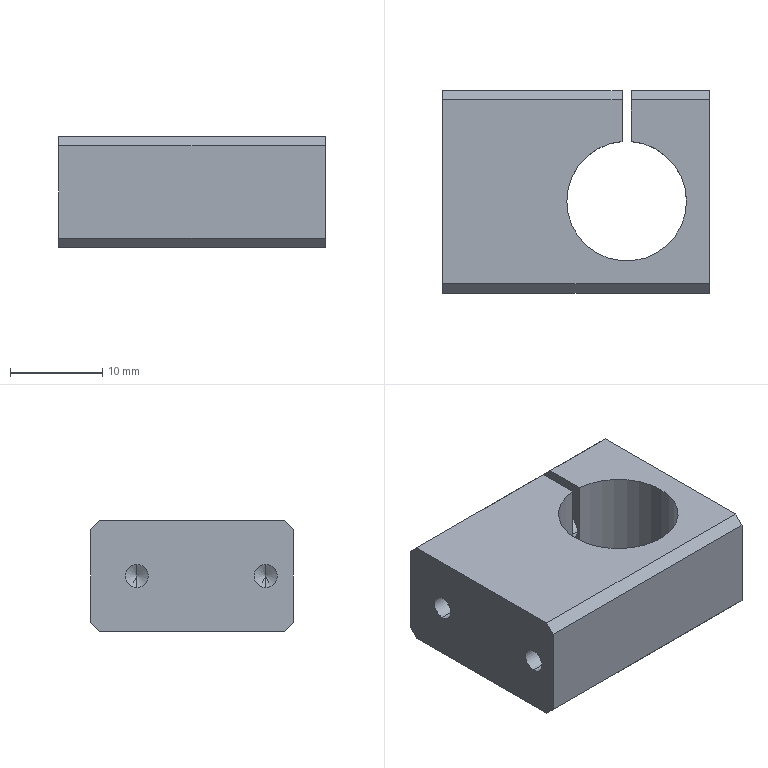NC program | NX | posted with a generic post | part box 29 x 22 x 12 mm
Whole program:
N10 G17 G21 G94 G90
(DRILLING_COPY_1 , TOOL : D6A45)
N12 T01 M6
N14 G54
N16 G17 G0 G90 X7.5 Y0. B0. C0. S5000 M3
N18 G43 Z30. H1
N20 G94 G81 G98 Z-1. F250. R3.
N22 G80
N24 G0 X7.5 Y0. Z30.
N26 M5
(DRILLING_COPY_1_COPY_COPY , TOOL : 2.5ZT)
N28 T12 M6
N30 G54
N32 G17 G0 G90 X7.5 Y0. B0. C0. S2000 M3
N34 G43 Z30. H12
N36 G94 G83 G98 Z-18.251 F150. Q2. R3.
N38 G80
N40 G0 X7.5 Y0. Z30.
N42 M5
(DRILLING_COPY_1_COPY , TOOL : 3.4ZT)
N44 T13 M6
N46 G54
N48 G17 G0 G90 X7.5 Y0. B0. C0. S2000 M3
N50 G43 Z30. H13
N52 G94 G83 G98 Z-10.021 F150. Q2. R3.
N54 G80
N56 G0 X7.5 Y0. Z30.
N58 M5
(HOLE_MILLING_1 , TOOL : D4)
N60 T04 M6
N62 G54
N64 G17 G0 G90 X7.5 Y0. B0. C0. S9500 M3
N66 G43 Z30. H4
N68 Z0.5
N70 G94 G3 X8. Y-0.5 R0.5 F1300.
N72 X8.5 Y0. R0.5
N74 X8.5 Y0. Z0.2 I-1. J0.
N76 X8.5 Y0. Z-0.1 I-1. J0.
N78 X8.5 Y0. Z-0.4 I-1. J0.
N80 X8.5 Y0. Z-0.7 I-1. J0.
N82 X8.5 Y0. Z-1. I-1. J0.
N84 X8.5 Y0. Z-1.3 I-1. J0.
N86 X8.5 Y0. Z-1.6 I-1. J0.
N88 X8.5 Y0. Z-1.9 I-1. J0.
N90 X8.5 Y0. Z-2.2 I-1. J0.
N92 X8.5 Y0. Z-2.5 I-1. J0.
N94 X8.5 Y0. Z-2.8 I-1. J0.
N96 X8.5 Y0. Z-3.1 I-1. J0.
N98 X8.5 Y0. Z-3.4 I-1. J0.
N100 X7.5 Y1. R1.
N102 X8.5 Y0. R-1.
N104 X8. Y0.5 R0.5
N106 X7.5 Y0. R0.5
N108 G0 Z30.
N110 M5
(11_COPY_COPY_COPY_COPY , TOOL : D6A45)
N112 T01 M6
N114 G54
N116 G17 G0 G90 X8.306 Y-0.241 B0. C0. S9500 M3
N118 G43 Z30. H1
N120 Z2.
N122 G94 G1 Z-1. F1000.
N124 X9.241 Y-0.52
N126 G3 X9.541 Y0. R0.6
N128 X7.5 Y2.041 R2.041
N130 X9.541 Y0. R-2.041
N132 X9.241 Y0.52 R0.6
N134 G1 X8.306 Y0.241
N136 Z2.
N138 G0 Z30.
N140 X-10.921 Y7.952
N142 Z2.
N144 G1 Z-1.
N146 X-10.52 Y7.259
N148 G3 X-10.001 Y6.959 R0.6
N150 G1 X10.001
N152 G2 X10.677 Y6.678 R0.957
N154 G1 X11.679 Y5.677
N156 G2 X11.959 Y5.001 R0.988
N158 G1 Y-5.001
N160 G2 X11.679 Y-5.677 R0.988
N162 G1 X10.677 Y-6.678
N164 G2 X10.001 Y-6.959 R0.957
N166 G1 X-10.001
N168 G2 X-10.677 Y-6.678 R0.957
N170 G1 X-11.678 Y-5.677
N172 G2 X-11.959 Y-5.001 R0.957
N174 G1 Y5.001
N176 G2 X-11.678 Y5.677 R0.957
N178 G1 X-10.677 Y6.678
N180 G2 X-10.001 Y6.959 R0.957
N182 G3 X-9.481 Y7.259 R0.6
N184 G1 X-8.961 Y8.159
N186 Z2.
N188 G0 Z30.
N190 M5
(CUTTERCOMP11 , TOOL : 2.3XYD)
N192 T11 M6
N194 G54
N196 G17 G0 G90 X7.5 Y0. B0. C0. S5000 M3
N198 G43 Z30. H11
N200 Z-7.936
N202 G42 G94 G1 X7.578 Y0.062 F850. D11
N204 X7.628 Y0.08 Z-7.957
N206 X7.675 Y0.052 Z-7.979
N208 X7.683 Y0. Z-8.
N210 G2 X7.683 Y0. Z-8.5 I-0.183 J0.
N212 X7.683 Y0. Z-9. I-0.183 J0.
N214 X7.683 Y0. Z-9.5 I-0.183 J0.
N216 X7.683 Y0. Z-10. I-0.183 J0.
N218 X7.683 Y0. Z-10.5 I-0.183 J0.
N220 X7.683 Y0. Z-11. I-0.183 J0.
N222 X7.683 Y0. Z-11.5 I-0.183 J0.
N224 X7.683 Y0. Z-12. I-0.183 J0.
N226 X7.683 Y0. Z-12.5 I-0.183 J0.
N228 X7.683 Y0. Z-13. I-0.183 J0.
N230 X7.683 Y0. Z-13.5 I-0.183 J0.
N232 X7.683 Y0. Z-14. I-0.183 J0.
N234 X7.683 Y0. Z-14.5 I-0.183 J0.
N236 X7.683 Y0. Z-15. I-0.183 J0.
N238 X7.683 Y0. Z-15.5 I-0.183 J0.
N240 X7.683 Y0. Z-16. I-0.183 J0.
N242 X7.683 Y0. Z-16.5 I-0.183 J0.
N244 X7.683 Y0. Z-17. I-0.183 J0.
N246 X7.683 Y0. Z-17.5 I-0.183 J0.
N248 G1 X7.675 Y-0.052 Z-17.521
N250 X7.628 Y-0.08 Z-17.543
N252 X7.578 Y-0.062 Z-17.564
N254 G40
N256 X7.5 Y0.
N258 G0 Z30.
N260 Z-7.913
N262 G42 G1 X7.555 Y0.084
N264 G2 X7.767 Y0. Z-8. R0.123
N266 X7.767 Y0. Z-8.5 I-0.267 J0.
N268 X7.767 Y0. Z-9. I-0.267 J0.
N270 X7.767 Y0. Z-9.5 I-0.267 J0.
N272 X7.767 Y0. Z-10. I-0.267 J0.
N274 X7.767 Y0. Z-10.5 I-0.267 J0.
N276 X7.767 Y0. Z-11. I-0.267 J0.
N278 X7.767 Y0. Z-11.5 I-0.267 J0.
N280 X7.767 Y0. Z-12. I-0.267 J0.
N282 X7.767 Y0. Z-12.5 I-0.267 J0.
N284 X7.767 Y0. Z-13. I-0.267 J0.
N286 X7.767 Y0. Z-13.5 I-0.267 J0.
N288 X7.767 Y0. Z-14. I-0.267 J0.
N290 X7.767 Y0. Z-14.5 I-0.267 J0.
N292 X7.767 Y0. Z-15. I-0.267 J0.
N294 X7.767 Y0. Z-15.5 I-0.267 J0.
N296 X7.767 Y0. Z-16. I-0.267 J0.
N298 X7.767 Y0. Z-16.5 I-0.267 J0.
N300 X7.767 Y0. Z-17. I-0.267 J0.
N302 X7.767 Y0. Z-17.5 I-0.267 J0.
N304 X7.555 Y-0.084 Z-17.587 R0.123
N306 G40
N308 G1 X7.5 Y0.
N310 G0 Z30.
N312 Z-7.901
N314 G42 G1 X7.539 Y0.092
N316 G2 X7.85 Y0. Z-8. R0.169
N318 X7.85 Y0. Z-8.5 I-0.35 J0.
N320 X7.85 Y0. Z-9. I-0.35 J0.
N322 X7.85 Y0. Z-9.5 I-0.35 J0.
N324 X7.85 Y0. Z-10. I-0.35 J0.
N326 X7.85 Y0. Z-10.5 I-0.35 J0.
N328 X7.85 Y0. Z-11. I-0.35 J0.
N330 X7.85 Y0. Z-11.5 I-0.35 J0.
N332 X7.85 Y0. Z-12. I-0.35 J0.
N334 X7.85 Y0. Z-12.5 I-0.35 J0.
N336 X7.85 Y0. Z-13. I-0.35 J0.
N338 X7.85 Y0. Z-13.5 I-0.35 J0.
N340 X7.85 Y0. Z-14. I-0.35 J0.
N342 X7.85 Y0. Z-14.5 I-0.35 J0.
N344 X7.85 Y0. Z-15. I-0.35 J0.
N346 X7.85 Y0. Z-15.5 I-0.35 J0.
N348 X7.85 Y0. Z-16. I-0.35 J0.
N350 X7.85 Y0. Z-16.5 I-0.35 J0.
N352 X7.85 Y0. Z-17. I-0.35 J0.
N354 X7.85 Y0. Z-17.5 I-0.35 J0.
N356 X7.539 Y-0.092 Z-17.599 R0.169
N358 G40
N360 G1 X7.5 Y0.
N362 G0 Z30.
N364 M5
N366 M2